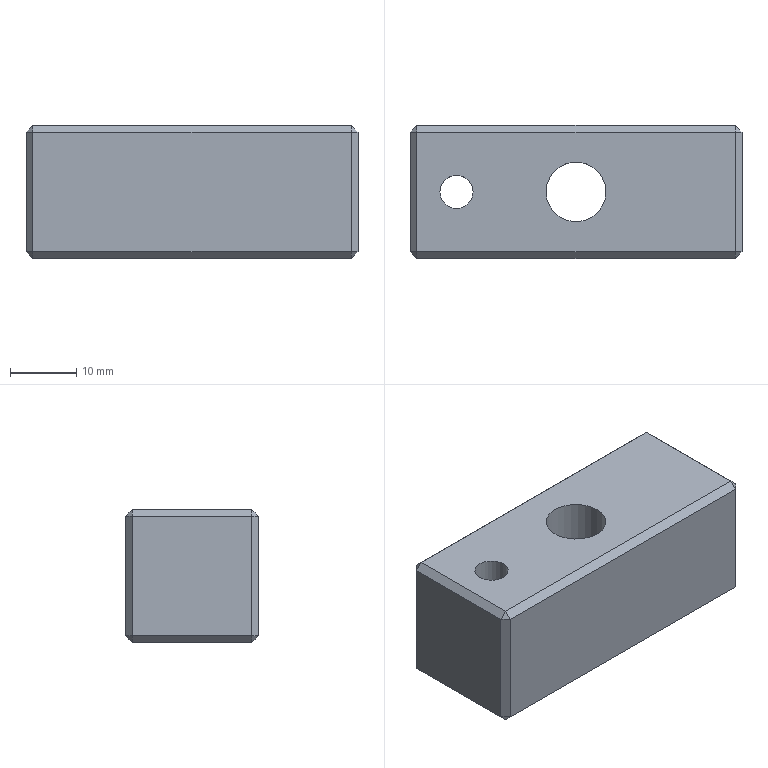Part | STEP file | gslz 2016.10.28-10_id1182_x_t | 1 solid | 81 faces | box 50 x 20 x 20 mm | volume 16939 mm3 | plane 63 | other 14 | cylinder 4 | commonest cylinder face diameters 5 x1 7 x1 9 x1 14 x1